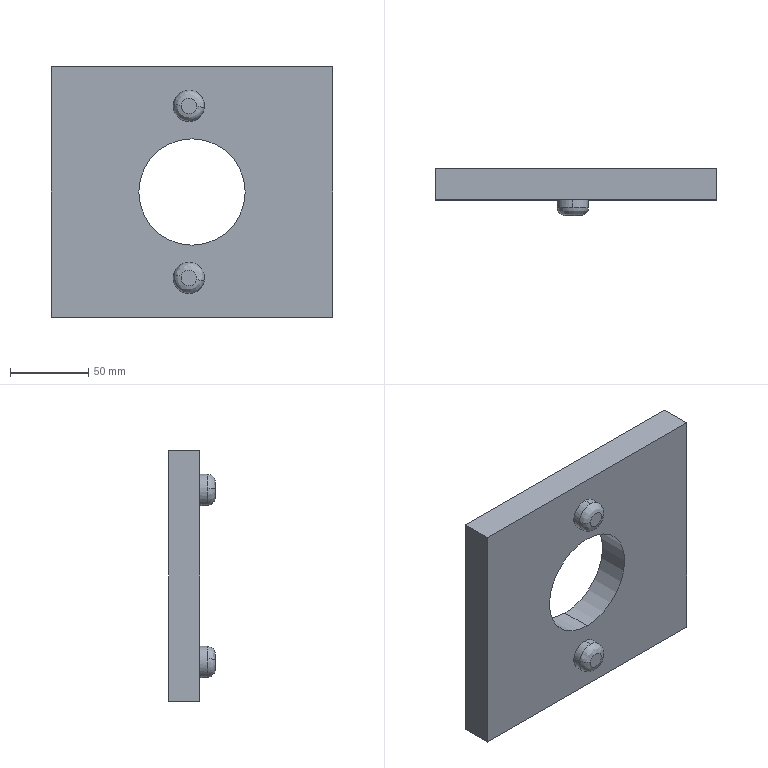Part | STEP file | leg control01_5 | 1 solid | 18 faces | box 180 x 30 x 160 mm | volume 509091 mm3 | plane 8 | cylinder 6 | spline 4 | commonest cylinder face diameters 20 x4 67.981 x2